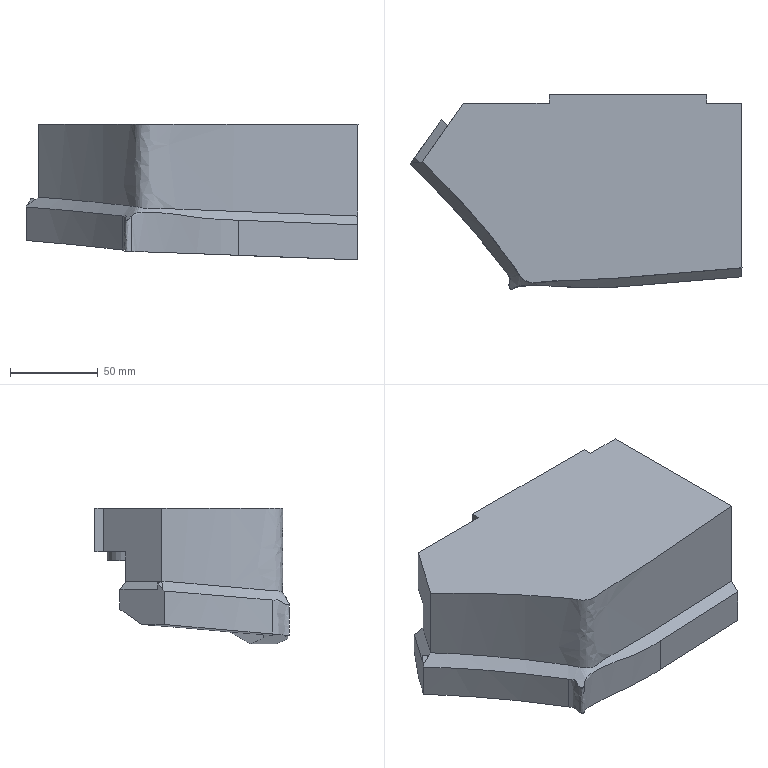Part | NX | features solid 2 | 1 solid | 35 faces | box 189.334 x 110.954 x 77.407 mm | volume 688111 mm3 | plane 16 | spline 14 | cylinder 5 | commonest cylinder face diameters 30 x5